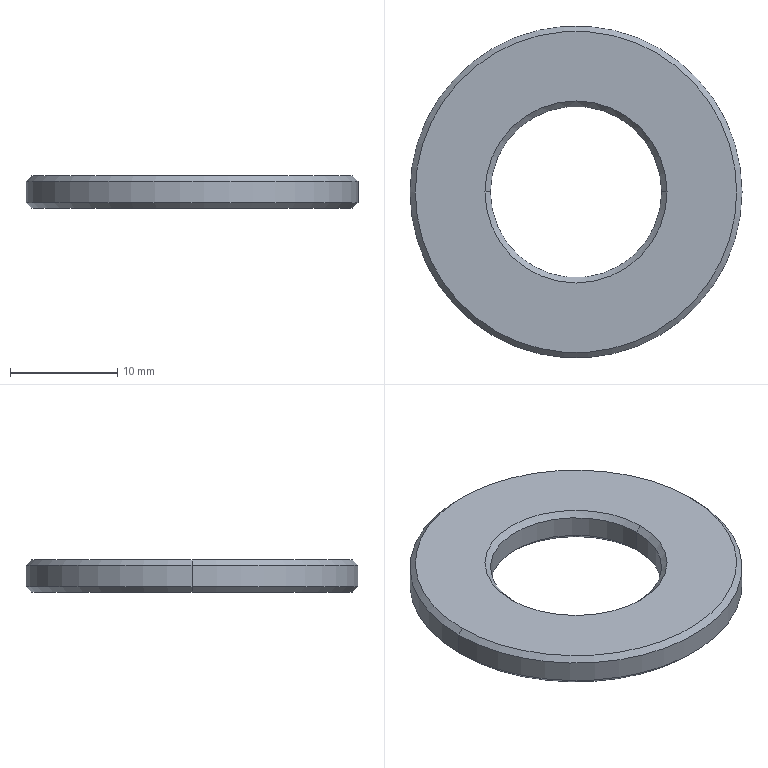Part | Creo | features DATUM PLANE 3, CHAMFER 1, COORDINATE SYSTEM 1, CURVE 1, PROTRUSION 1 | 1 solid | 14 faces | box 31 x 31 x 3 mm | volume 1624 mm3 | cone 8 | cylinder 4 | plane 2 | commonest cylinder face diameters 16 x2 31 x2
STEP:
#1=CARTESIAN_POINT('',(0.,0.,0.));
#2=DIRECTION('',(0.,0.,1.));
#3=DIRECTION('',(1.,0.,0.));
#4=AXIS2_PLACEMENT_3D('',#1,#2,#3);
#5=CARTESIAN_POINT('',(-15.,0.,0.));
#6=VERTEX_POINT('',#5);
#7=CARTESIAN_POINT('',(15.,0.,0.));
#8=VERTEX_POINT('',#7);
#9=CARTESIAN_POINT('',(0.,0.,0.));
#10=DIRECTION('',(0.,0.,-1.));
#11=DIRECTION('',(-1.,0.,0.));
#12=AXIS2_PLACEMENT_3D('',#9,#10,#11);
#13=CIRCLE('',#12,15.);
#14=EDGE_CURVE('',#6,#8,#13,.T.);
#15=ORIENTED_EDGE('',*,*,#14,.F.);
#16=CARTESIAN_POINT('',(0.,0.,0.));
#17=DIRECTION('',(0.,0.,-1.));
#18=DIRECTION('',(1.,0.,0.));
#19=AXIS2_PLACEMENT_3D('',#16,#17,#18);
#20=CIRCLE('',#19,15.);
#21=EDGE_CURVE('',#8,#6,#20,.T.);
#22=ORIENTED_EDGE('',*,*,#21,.F.);
#23=EDGE_LOOP('',(#15,#22));
#24=FACE_OUTER_BOUND('',#23,.F.);
#25=CARTESIAN_POINT('',(-8.5,0.,0.));
#26=VERTEX_POINT('',#25);
#27=CARTESIAN_POINT('',(8.5,0.,0.));
#28=VERTEX_POINT('',#27);
#29=CARTESIAN_POINT('',(0.,0.,0.));
#30=DIRECTION('',(0.,0.,1.));
#31=DIRECTION('',(-1.,0.,0.));
#32=AXIS2_PLACEMENT_3D('',#29,#30,#31);
#33=CIRCLE('',#32,8.5);
#34=EDGE_CURVE('',#26,#28,#33,.T.);
#35=ORIENTED_EDGE('',*,*,#34,.F.);
#36=CARTESIAN_POINT('',(0.,0.,0.));
#37=DIRECTION('',(0.,0.,1.));
#38=DIRECTION('',(1.,0.,0.));
#39=AXIS2_PLACEMENT_3D('',#36,#37,#38);
#40=CIRCLE('',#39,8.5);
#41=EDGE_CURVE('',#28,#26,#40,.T.);
#42=ORIENTED_EDGE('',*,*,#41,.F.);
#43=EDGE_LOOP('',(#35,#42));
#44=FACE_BOUND('',#43,.F.);
#45=CARTESIAN_POINT('',(0.,0.,0.));
#46=DIRECTION('',(0.,0.,1.));
#47=DIRECTION('',(1.,0.,0.));
#48=AXIS2_PLACEMENT_3D('',#45,#46,#47);
#49=PLANE('',#48);
#50=ADVANCED_FACE('',(#24,#44),#49,.F.);
#51=ORIENTED_EDGE('',*,*,#14,.T.);
#52=CARTESIAN_POINT('',(15.5,0.,0.5));
#53=VERTEX_POINT('',#52);
#54=CARTESIAN_POINT('',(15.,0.000000002,0.));
#55=DIRECTION('',(0.7071,-0.000000001,0.7071));
#56=VECTOR('',#55,0.7071);
#57=LINE('',#54,#56);
#58=EDGE_CURVE('',#8,#53,#57,.T.);
#59=ORIENTED_EDGE('',*,*,#58,.T.);
#60=CARTESIAN_POINT('',(-15.5,0.,0.5));
#61=VERTEX_POINT('',#60);
#62=CARTESIAN_POINT('',(0.,0.,0.5));
#63=DIRECTION('',(0.,0.,-1.));
#64=DIRECTION('',(-1.,0.,0.));
#65=AXIS2_PLACEMENT_3D('',#62,#63,#64);
#66=CIRCLE('',#65,15.5);
#67=EDGE_CURVE('',#61,#53,#66,.T.);
#68=ORIENTED_EDGE('',*,*,#67,.F.);
#69=CARTESIAN_POINT('',(-15.,-0.000000002,0.));
#70=DIRECTION('',(-0.7071,0.000000001,0.7071));
#71=VECTOR('',#70,0.7071);
#72=LINE('',#69,#71);
#73=EDGE_CURVE('',#6,#61,#72,.T.);
#74=ORIENTED_EDGE('',*,*,#73,.F.);
#75=EDGE_LOOP('',(#51,#59,#68,#74));
#76=FACE_OUTER_BOUND('',#75,.F.);
#77=CARTESIAN_POINT('',(0.,0.,0.25));
#78=DIRECTION('',(0.,0.,1.));
#79=DIRECTION('',(0.,-1.,0.));
#80=AXIS2_PLACEMENT_3D('',#77,#78,#79);
#81=CONICAL_SURFACE('',#80,15.25,45.);
#82=ADVANCED_FACE('',(#76),#81,.T.);
#83=ORIENTED_EDGE('',*,*,#21,.T.);
#84=ORIENTED_EDGE('',*,*,#73,.T.);
#85=CARTESIAN_POINT('',(0.,0.,0.5));
#86=DIRECTION('',(0.,0.,-1.));
#87=DIRECTION('',(1.,0.,0.));
#88=AXIS2_PLACEMENT_3D('',#85,#86,#87);
#89=CIRCLE('',#88,15.5);
#90=EDGE_CURVE('',#53,#61,#89,.T.);
#91=ORIENTED_EDGE('',*,*,#90,.F.);
#92=ORIENTED_EDGE('',*,*,#58,.F.);
#93=EDGE_LOOP('',(#83,#84,#91,#92));
#94=FACE_OUTER_BOUND('',#93,.F.);
#95=CARTESIAN_POINT('',(0.,0.,0.25));
#96=DIRECTION('',(0.,0.,1.));
#97=DIRECTION('',(0.,-1.,0.));
#98=AXIS2_PLACEMENT_3D('',#95,#96,#97);
#99=CONICAL_SURFACE('',#98,15.25,45.);
#100=ADVANCED_FACE('',(#94),#99,.T.);
#101=CARTESIAN_POINT('',(-15.5,0.,2.5));
#102=VERTEX_POINT('',#101);
#103=CARTESIAN_POINT('',(15.5,0.,2.5));
#104=VERTEX_POINT('',#103);
#105=CARTESIAN_POINT('',(0.,0.,2.5));
#106=DIRECTION('',(0.,0.,1.));
#107=DIRECTION('',(-1.,0.,0.));
#108=AXIS2_PLACEMENT_3D('',#105,#106,#107);
#109=CIRCLE('',#108,15.5);
#110=EDGE_CURVE('',#102,#104,#109,.T.);
#111=ORIENTED_EDGE('',*,*,#110,.T.);
#112=CARTESIAN_POINT('',(15.5,0.000000002,0.5));
#113=DIRECTION('',(0.,0.,1.));
#114=VECTOR('',#113,2.);
#115=LINE('',#112,#114);
#116=EDGE_CURVE('',#53,#104,#115,.T.);
#117=ORIENTED_EDGE('',*,*,#116,.F.);
#118=ORIENTED_EDGE('',*,*,#90,.T.);
#119=CARTESIAN_POINT('',(-15.5,-0.000000002,0.5));
#120=DIRECTION('',(0.,0.,1.));
#121=VECTOR('',#120,2.);
#122=LINE('',#119,#121);
#123=EDGE_CURVE('',#61,#102,#122,.T.);
#124=ORIENTED_EDGE('',*,*,#123,.T.);
#125=EDGE_LOOP('',(#111,#117,#118,#124));
#126=FACE_OUTER_BOUND('',#125,.F.);
#127=CARTESIAN_POINT('',(0.,0.,0.));
#128=DIRECTION('',(0.,0.,1.));
#129=DIRECTION('',(1.,0.,0.));
#130=AXIS2_PLACEMENT_3D('',#127,#128,#129);
#131=CYLINDRICAL_SURFACE('',#130,15.5);
#132=ADVANCED_FACE('',(#126),#131,.T.);
#133=CARTESIAN_POINT('',(-15.,0.,3.));
#134=VERTEX_POINT('',#133);
#135=CARTESIAN_POINT('',(15.,0.,3.));
#136=VERTEX_POINT('',#135);
#137=CARTESIAN_POINT('',(0.,0.,3.));
#138=DIRECTION('',(0.,0.,1.));
#139=DIRECTION('',(-1.,0.,0.));
#140=AXIS2_PLACEMENT_3D('',#137,#138,#139);
#141=CIRCLE('',#140,15.);
#142=EDGE_CURVE('',#134,#136,#141,.T.);
#143=ORIENTED_EDGE('',*,*,#142,.T.);
#144=CARTESIAN_POINT('',(15.,0.000000002,3.));
#145=DIRECTION('',(0.7071,-0.000000001,-0.7071));
#146=VECTOR('',#145,0.7071);
#147=LINE('',#144,#146);
#148=EDGE_CURVE('',#136,#104,#147,.T.);
#149=ORIENTED_EDGE('',*,*,#148,.T.);
#150=ORIENTED_EDGE('',*,*,#110,.F.);
#151=CARTESIAN_POINT('',(-15.,-0.000000002,3.));
#152=DIRECTION('',(-0.7071,0.000000001,-0.7071));
#153=VECTOR('',#152,0.7071);
#154=LINE('',#151,#153);
#155=EDGE_CURVE('',#134,#102,#154,.T.);
#156=ORIENTED_EDGE('',*,*,#155,.F.);
#157=EDGE_LOOP('',(#143,#149,#150,#156));
#158=FACE_OUTER_BOUND('',#157,.F.);
#159=CARTESIAN_POINT('',(0.,0.,2.75));
#160=DIRECTION('',(0.,0.,-1.));
#161=DIRECTION('',(0.,-1.,0.));
#162=AXIS2_PLACEMENT_3D('',#159,#160,#161);
#163=CONICAL_SURFACE('',#162,15.25,45.);
#164=ADVANCED_FACE('',(#158),#163,.T.);
#165=CARTESIAN_POINT('',(0.,0.,3.));
#166=DIRECTION('',(0.,0.,1.));
#167=DIRECTION('',(1.,0.,0.));
#168=AXIS2_PLACEMENT_3D('',#165,#166,#167);
#169=CIRCLE('',#168,15.);
#170=EDGE_CURVE('',#136,#134,#169,.T.);
#171=ORIENTED_EDGE('',*,*,#170,.F.);
#172=ORIENTED_EDGE('',*,*,#142,.F.);
#173=EDGE_LOOP('',(#171,#172));
#174=FACE_OUTER_BOUND('',#173,.F.);
#175=CARTESIAN_POINT('',(8.5,0.,3.));
#176=VERTEX_POINT('',#175);
#177=CARTESIAN_POINT('',(-8.5,0.,3.));
#178=VERTEX_POINT('',#177);
#179=CARTESIAN_POINT('',(0.,0.,3.));
#180=DIRECTION('',(0.,0.,-1.));
#181=DIRECTION('',(1.,0.,0.));
#182=AXIS2_PLACEMENT_3D('',#179,#180,#181);
#183=CIRCLE('',#182,8.5);
#184=EDGE_CURVE('',#176,#178,#183,.T.);
#185=ORIENTED_EDGE('',*,*,#184,.F.);
#186=CARTESIAN_POINT('',(0.,0.,3.));
#187=DIRECTION('',(0.,0.,-1.));
#188=DIRECTION('',(-1.,0.,0.));
#189=AXIS2_PLACEMENT_3D('',#186,#187,#188);
#190=CIRCLE('',#189,8.5);
#191=EDGE_CURVE('',#178,#176,#190,.T.);
#192=ORIENTED_EDGE('',*,*,#191,.F.);
#193=EDGE_LOOP('',(#185,#192));
#194=FACE_BOUND('',#193,.F.);
#195=CARTESIAN_POINT('',(0.,0.,3.));
#196=DIRECTION('',(0.,0.,1.));
#197=DIRECTION('',(1.,0.,0.));
#198=AXIS2_PLACEMENT_3D('',#195,#196,#197);
#199=PLANE('',#198);
#200=ADVANCED_FACE('',(#174,#194),#199,.T.);
#201=ORIENTED_EDGE('',*,*,#170,.T.);
#202=ORIENTED_EDGE('',*,*,#155,.T.);
#203=CARTESIAN_POINT('',(0.,0.,2.5));
#204=DIRECTION('',(0.,0.,1.));
#205=DIRECTION('',(1.,0.,0.));
#206=AXIS2_PLACEMENT_3D('',#203,#204,#205);
#207=CIRCLE('',#206,15.5);
#208=EDGE_CURVE('',#104,#102,#207,.T.);
#209=ORIENTED_EDGE('',*,*,#208,.F.);
#210=ORIENTED_EDGE('',*,*,#148,.F.);
#211=EDGE_LOOP('',(#201,#202,#209,#210));
#212=FACE_OUTER_BOUND('',#211,.F.);
#213=CARTESIAN_POINT('',(0.,0.,2.75));
#214=DIRECTION('',(0.,0.,-1.));
#215=DIRECTION('',(0.,-1.,0.));
#216=AXIS2_PLACEMENT_3D('',#213,#214,#215);
#217=CONICAL_SURFACE('',#216,15.25,45.);
#218=ADVANCED_FACE('',(#212),#217,.T.);
#219=ORIENTED_EDGE('',*,*,#208,.T.);
#220=ORIENTED_EDGE('',*,*,#123,.F.);
#221=ORIENTED_EDGE('',*,*,#67,.T.);
#222=ORIENTED_EDGE('',*,*,#116,.T.);
#223=EDGE_LOOP('',(#219,#220,#221,#222));
#224=FACE_OUTER_BOUND('',#223,.F.);
#225=CARTESIAN_POINT('',(0.,0.,0.));
#226=DIRECTION('',(0.,0.,1.));
#227=DIRECTION('',(1.,0.,0.));
#228=AXIS2_PLACEMENT_3D('',#225,#226,#227);
#229=CYLINDRICAL_SURFACE('',#228,15.5);
#230=ADVANCED_FACE('',(#224),#229,.T.);
#231=ORIENTED_EDGE('',*,*,#184,.T.);
#232=CARTESIAN_POINT('',(-8.,0.,2.5));
#233=VERTEX_POINT('',#232);
#234=CARTESIAN_POINT('',(-8.5,-0.000000005,3.));
#235=DIRECTION('',(0.7071,0.000000002,-0.7071));
#236=VECTOR('',#235,0.7071);
#237=LINE('',#234,#236);
#238=EDGE_CURVE('',#178,#233,#237,.T.);
#239=ORIENTED_EDGE('',*,*,#238,.T.);
#240=CARTESIAN_POINT('',(8.,0.,2.5));
#241=VERTEX_POINT('',#240);
#242=CARTESIAN_POINT('',(0.,0.,2.5));
#243=DIRECTION('',(0.,0.,-1.));
#244=DIRECTION('',(1.,0.,0.));
#245=AXIS2_PLACEMENT_3D('',#242,#243,#244);
#246=CIRCLE('',#245,8.);
#247=EDGE_CURVE('',#241,#233,#246,.T.);
#248=ORIENTED_EDGE('',*,*,#247,.F.);
#249=CARTESIAN_POINT('',(8.5,0.000000005,3.));
#250=DIRECTION('',(-0.7071,-0.000000002,-0.7071));
#251=VECTOR('',#250,0.7071);
#252=LINE('',#249,#251);
#253=EDGE_CURVE('',#176,#241,#252,.T.);
#254=ORIENTED_EDGE('',*,*,#253,.F.);
#255=EDGE_LOOP('',(#231,#239,#248,#254));
#256=FACE_OUTER_BOUND('',#255,.F.);
#257=CARTESIAN_POINT('',(0.,0.,2.75));
#258=DIRECTION('',(0.,0.,1.));
#259=DIRECTION('',(0.,-1.,0.));
#260=AXIS2_PLACEMENT_3D('',#257,#258,#259);
#261=CONICAL_SURFACE('',#260,8.25,45.);
#262=ADVANCED_FACE('',(#256),#261,.F.);
#263=ORIENTED_EDGE('',*,*,#191,.T.);
#264=ORIENTED_EDGE('',*,*,#253,.T.);
#265=CARTESIAN_POINT('',(0.,0.,2.5));
#266=DIRECTION('',(0.,0.,-1.));
#267=DIRECTION('',(-1.,0.,0.));
#268=AXIS2_PLACEMENT_3D('',#265,#266,#267);
#269=CIRCLE('',#268,8.);
#270=EDGE_CURVE('',#233,#241,#269,.T.);
#271=ORIENTED_EDGE('',*,*,#270,.F.);
#272=ORIENTED_EDGE('',*,*,#238,.F.);
#273=EDGE_LOOP('',(#263,#264,#271,#272));
#274=FACE_OUTER_BOUND('',#273,.F.);
#275=CARTESIAN_POINT('',(0.,0.,2.75));
#276=DIRECTION('',(0.,0.,1.));
#277=DIRECTION('',(0.,-1.,0.));
#278=AXIS2_PLACEMENT_3D('',#275,#276,#277);
#279=CONICAL_SURFACE('',#278,8.25,45.);
#280=ADVANCED_FACE('',(#274),#279,.F.);
#281=CARTESIAN_POINT('',(8.,0.,0.5));
#282=VERTEX_POINT('',#281);
#283=CARTESIAN_POINT('',(-8.,0.,0.5));
#284=VERTEX_POINT('',#283);
#285=CARTESIAN_POINT('',(0.,0.,0.5));
#286=DIRECTION('',(0.,0.,1.));
#287=DIRECTION('',(1.,0.,0.));
#288=AXIS2_PLACEMENT_3D('',#285,#286,#287);
#289=CIRCLE('',#288,8.);
#290=EDGE_CURVE('',#282,#284,#289,.T.);
#291=ORIENTED_EDGE('',*,*,#290,.T.);
#292=CARTESIAN_POINT('',(-8.,-0.000000003,0.5));
#293=DIRECTION('',(0.,0.,1.));
#294=VECTOR('',#293,2.);
#295=LINE('',#292,#294);
#296=EDGE_CURVE('',#284,#233,#295,.T.);
#297=ORIENTED_EDGE('',*,*,#296,.T.);
#298=ORIENTED_EDGE('',*,*,#270,.T.);
#299=CARTESIAN_POINT('',(8.,0.000000003,0.5));
#300=DIRECTION('',(0.,0.,1.));
#301=VECTOR('',#300,2.);
#302=LINE('',#299,#301);
#303=EDGE_CURVE('',#282,#241,#302,.T.);
#304=ORIENTED_EDGE('',*,*,#303,.F.);
#305=EDGE_LOOP('',(#291,#297,#298,#304));
#306=FACE_OUTER_BOUND('',#305,.F.);
#307=CARTESIAN_POINT('',(0.,0.,0.));
#308=DIRECTION('',(0.,0.,1.));
#309=DIRECTION('',(1.,0.,0.));
#310=AXIS2_PLACEMENT_3D('',#307,#308,#309);
#311=CYLINDRICAL_SURFACE('',#310,8.);
#312=ADVANCED_FACE('',(#306),#311,.F.);
#313=ORIENTED_EDGE('',*,*,#41,.T.);
#314=CARTESIAN_POINT('',(-8.5,-0.000000005,0.));
#315=DIRECTION('',(0.7071,0.000000002,0.7071));
#316=VECTOR('',#315,0.7071);
#317=LINE('',#314,#316);
#318=EDGE_CURVE('',#26,#284,#317,.T.);
#319=ORIENTED_EDGE('',*,*,#318,.T.);
#320=ORIENTED_EDGE('',*,*,#290,.F.);
#321=CARTESIAN_POINT('',(8.5,0.000000005,0.));
#322=DIRECTION('',(-0.7071,-0.000000002,0.7071));
#323=VECTOR('',#322,0.7071);
#324=LINE('',#321,#323);
#325=EDGE_CURVE('',#28,#282,#324,.T.);
#326=ORIENTED_EDGE('',*,*,#325,.F.);
#327=EDGE_LOOP('',(#313,#319,#320,#326));
#328=FACE_OUTER_BOUND('',#327,.F.);
#329=CARTESIAN_POINT('',(0.,0.,0.25));
#330=DIRECTION('',(0.,0.,-1.));
#331=DIRECTION('',(0.,-1.,0.));
#332=AXIS2_PLACEMENT_3D('',#329,#330,#331);
#333=CONICAL_SURFACE('',#332,8.25,45.);
#334=ADVANCED_FACE('',(#328),#333,.F.);
#335=ORIENTED_EDGE('',*,*,#34,.T.);
#336=ORIENTED_EDGE('',*,*,#325,.T.);
#337=CARTESIAN_POINT('',(0.,0.,0.5));
#338=DIRECTION('',(0.,0.,1.));
#339=DIRECTION('',(-1.,0.,0.));
#340=AXIS2_PLACEMENT_3D('',#337,#338,#339);
#341=CIRCLE('',#340,8.);
#342=EDGE_CURVE('',#284,#282,#341,.T.);
#343=ORIENTED_EDGE('',*,*,#342,.F.);
#344=ORIENTED_EDGE('',*,*,#318,.F.);
#345=EDGE_LOOP('',(#335,#336,#343,#344));
#346=FACE_OUTER_BOUND('',#345,.F.);
#347=CARTESIAN_POINT('',(0.,0.,0.25));
#348=DIRECTION('',(0.,0.,-1.));
#349=DIRECTION('',(0.,-1.,0.));
#350=AXIS2_PLACEMENT_3D('',#347,#348,#349);
#351=CONICAL_SURFACE('',#350,8.25,45.);
#352=ADVANCED_FACE('',(#346),#351,.F.);
#353=ORIENTED_EDGE('',*,*,#342,.T.);
#354=ORIENTED_EDGE('',*,*,#303,.T.);
#355=ORIENTED_EDGE('',*,*,#247,.T.);
#356=ORIENTED_EDGE('',*,*,#296,.F.);
#357=EDGE_LOOP('',(#353,#354,#355,#356));
#358=FACE_OUTER_BOUND('',#357,.F.);
#359=CARTESIAN_POINT('',(0.,0.,0.));
#360=DIRECTION('',(0.,0.,1.));
#361=DIRECTION('',(1.,0.,0.));
#362=AXIS2_PLACEMENT_3D('',#359,#360,#361);
#363=CYLINDRICAL_SURFACE('',#362,8.);
#364=ADVANCED_FACE('',(#358),#363,.F.);
#365=CLOSED_SHELL('',(#50,#82,#100,#132,#164,#200,#218,#230,#262,#280,#312,#334,#352,#364));
#366=MANIFOLD_SOLID_BREP('',#365);
#367=(LENGTH_UNIT()NAMED_UNIT(*)SI_UNIT(.MILLI.,.METRE.));
#368=UNCERTAINTY_MEASURE_WITH_UNIT(LENGTH_MEASURE(0.004396),#367,'','');
#369=(NAMED_UNIT(*)PLANE_ANGLE_UNIT()SI_UNIT($,.RADIAN.));
#370=PLANE_ANGLE_MEASURE_WITH_UNIT(PLANE_ANGLE_MEASURE(0.01745),#369);
#371=(CONVERSION_BASED_UNIT('DEGREE',#370)NAMED_UNIT(*)PLANE_ANGLE_UNIT());
#372=(NAMED_UNIT(*)SI_UNIT($,.STERADIAN.)SOLID_ANGLE_UNIT());
#373=(GEOMETRIC_REPRESENTATION_CONTEXT(3)GLOBAL_UNCERTAINTY_ASSIGNED_CONTEXT((#368))GLOBAL_UNIT_ASSIGNED_CONTEXT((#367,#371,#372))REPRESENTATION_CONTEXT('',''));
#374=ADVANCED_BREP_SHAPE_REPRESENTATION('',(#4,#366),#373);